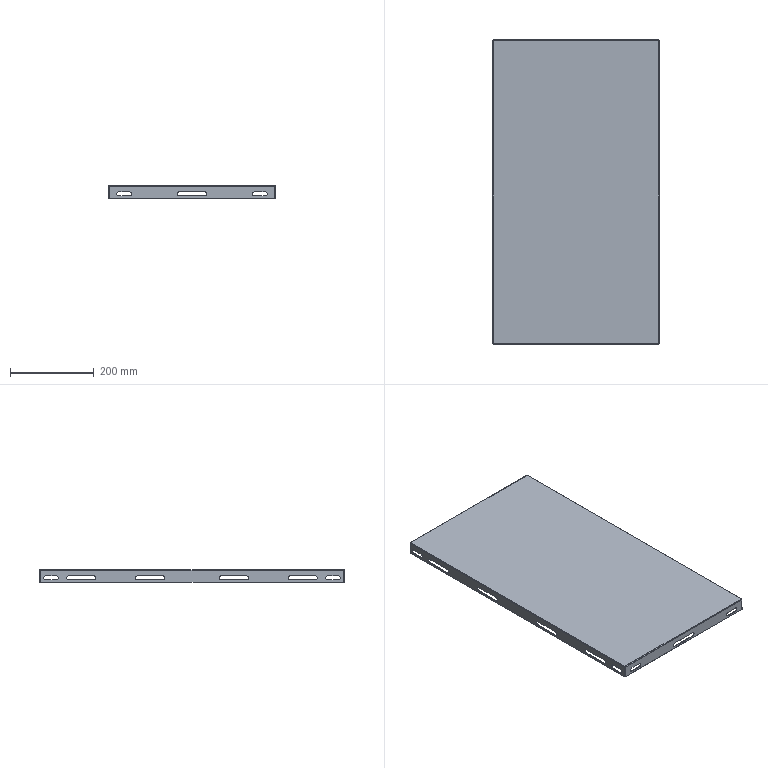Part | SolidWorks | features ICE 2, EdgeFlange 1, FlatPattern 1, SMBaseFlange 1, SheetMetal 1 | 1 solid | 110 faces | box 399 x 729 x 30 mm | volume 516047 mm3 | plane 58 | cylinder 44 | spline 8 | commonest cylinder face diameters 10 x36 1 x4 4 x4